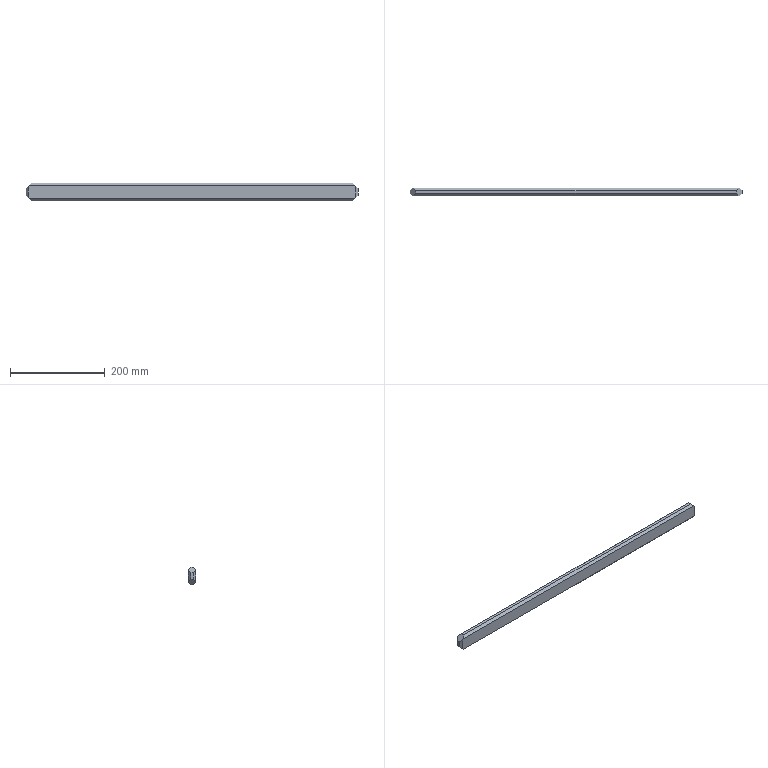Part | SolidWorks | features Chamfer 2, FlatPattern 1, SMBaseFlange 1, SheetMetal 1 | 1 solid | 18 faces | box 700 x 16 x 37 mm | volume 375009 mm3 | plane 18
STEP:
#1=CARTESIAN_POINT('',(0.,-11.,-25.));
#2=VERTEX_POINT('',#1);
#3=CARTESIAN_POINT('',(0.,-11.,-12.));
#4=VERTEX_POINT('',#3);
#5=CARTESIAN_POINT('',(0.,-11.,0.));
#6=DIRECTION('',(0.,0.,1.));
#7=VECTOR('',#6,1000.);
#8=LINE('',#5,#7);
#9=EDGE_CURVE('',#2,#4,#8,.T.);
#10=ORIENTED_EDGE('',*,*,#9,.T.);
#11=CARTESIAN_POINT('',(0.,-5.,-12.));
#12=VERTEX_POINT('',#11);
#13=CARTESIAN_POINT('',(0.,-16.,-12.));
#14=DIRECTION('',(0.,1.,0.));
#15=VECTOR('',#14,1000.);
#16=LINE('',#13,#15);
#17=EDGE_CURVE('',#4,#12,#16,.T.);
#18=ORIENTED_EDGE('',*,*,#17,.T.);
#19=CARTESIAN_POINT('',(0.,-5.,-25.));
#20=VERTEX_POINT('',#19);
#21=CARTESIAN_POINT('',(0.,-5.,-37.));
#22=DIRECTION('',(0.,0.,-1.));
#23=VECTOR('',#22,1000.);
#24=LINE('',#21,#23);
#25=EDGE_CURVE('',#12,#20,#24,.T.);
#26=ORIENTED_EDGE('',*,*,#25,.T.);
#27=CARTESIAN_POINT('',(0.,-16.,-25.));
#28=DIRECTION('',(0.,-1.,0.));
#29=VECTOR('',#28,1000.);
#30=LINE('',#27,#29);
#31=EDGE_CURVE('',#20,#2,#30,.T.);
#32=ORIENTED_EDGE('',*,*,#31,.T.);
#33=EDGE_LOOP('',(#10,#18,#26,#32));
#34=FACE_OUTER_BOUND('',#33,.T.);
#35=CARTESIAN_POINT('',(0.,-16.,0.));
#36=DIRECTION('',(-1.,0.,0.));
#37=DIRECTION('',(0.,0.,1.));
#38=AXIS2_PLACEMENT_3D('',#35,#36,#37);
#39=PLANE('',#38);
#40=ADVANCED_FACE('',(#34),#39,.T.);
#41=CARTESIAN_POINT('',(12.,-5.,-37.));
#42=VERTEX_POINT('',#41);
#43=CARTESIAN_POINT('',(688.,-5.,-37.));
#44=VERTEX_POINT('',#43);
#45=CARTESIAN_POINT('',(700.,-5.,-37.));
#46=DIRECTION('',(1.,0.,0.));
#47=VECTOR('',#46,1000.);
#48=LINE('',#45,#47);
#49=EDGE_CURVE('',#42,#44,#48,.T.);
#50=ORIENTED_EDGE('',*,*,#49,.T.);
#51=CARTESIAN_POINT('',(688.,-11.,-37.));
#52=VERTEX_POINT('',#51);
#53=CARTESIAN_POINT('',(688.,-16.,-37.));
#54=DIRECTION('',(0.,-1.,0.));
#55=VECTOR('',#54,1000.);
#56=LINE('',#53,#55);
#57=EDGE_CURVE('',#44,#52,#56,.T.);
#58=ORIENTED_EDGE('',*,*,#57,.T.);
#59=CARTESIAN_POINT('',(12.,-11.,-37.));
#60=VERTEX_POINT('',#59);
#61=CARTESIAN_POINT('',(0.,-11.,-37.));
#62=DIRECTION('',(-1.,0.,0.));
#63=VECTOR('',#62,1000.);
#64=LINE('',#61,#63);
#65=EDGE_CURVE('',#52,#60,#64,.T.);
#66=ORIENTED_EDGE('',*,*,#65,.T.);
#67=CARTESIAN_POINT('',(12.,-16.,-37.));
#68=DIRECTION('',(0.,1.,0.));
#69=VECTOR('',#68,1000.);
#70=LINE('',#67,#69);
#71=EDGE_CURVE('',#60,#42,#70,.T.);
#72=ORIENTED_EDGE('',*,*,#71,.T.);
#73=EDGE_LOOP('',(#50,#58,#66,#72));
#74=FACE_OUTER_BOUND('',#73,.T.);
#75=CARTESIAN_POINT('',(0.,-16.,-37.));
#76=DIRECTION('',(0.,0.,-1.));
#77=DIRECTION('',(-1.,0.,0.));
#78=AXIS2_PLACEMENT_3D('',#75,#76,#77);
#79=PLANE('',#78);
#80=ADVANCED_FACE('',(#74),#79,.T.);
#81=CARTESIAN_POINT('',(700.,-5.,-25.));
#82=VERTEX_POINT('',#81);
#83=CARTESIAN_POINT('',(700.,-5.,-12.));
#84=VERTEX_POINT('',#83);
#85=CARTESIAN_POINT('',(700.,-5.,0.));
#86=DIRECTION('',(0.,0.,1.));
#87=VECTOR('',#86,1000.);
#88=LINE('',#85,#87);
#89=EDGE_CURVE('',#82,#84,#88,.T.);
#90=ORIENTED_EDGE('',*,*,#89,.T.);
#91=CARTESIAN_POINT('',(700.,-11.,-12.));
#92=VERTEX_POINT('',#91);
#93=CARTESIAN_POINT('',(700.,-16.,-12.));
#94=DIRECTION('',(0.,-1.,0.));
#95=VECTOR('',#94,1000.);
#96=LINE('',#93,#95);
#97=EDGE_CURVE('',#84,#92,#96,.T.);
#98=ORIENTED_EDGE('',*,*,#97,.T.);
#99=CARTESIAN_POINT('',(700.,-11.,-25.));
#100=VERTEX_POINT('',#99);
#101=CARTESIAN_POINT('',(700.,-11.,0.));
#102=DIRECTION('',(0.,0.,-1.));
#103=VECTOR('',#102,1000.);
#104=LINE('',#101,#103);
#105=EDGE_CURVE('',#92,#100,#104,.T.);
#106=ORIENTED_EDGE('',*,*,#105,.T.);
#107=CARTESIAN_POINT('',(700.,-16.,-25.));
#108=DIRECTION('',(0.,1.,0.));
#109=VECTOR('',#108,1000.);
#110=LINE('',#107,#109);
#111=EDGE_CURVE('',#100,#82,#110,.T.);
#112=ORIENTED_EDGE('',*,*,#111,.T.);
#113=EDGE_LOOP('',(#90,#98,#106,#112));
#114=FACE_OUTER_BOUND('',#113,.T.);
#115=CARTESIAN_POINT('',(700.,-16.,0.));
#116=DIRECTION('',(1.,0.,0.));
#117=DIRECTION('',(0.,0.,-1.));
#118=AXIS2_PLACEMENT_3D('',#115,#116,#117);
#119=PLANE('',#118);
#120=ADVANCED_FACE('',(#114),#119,.T.);
#121=CARTESIAN_POINT('',(12.,-11.,0.));
#122=VERTEX_POINT('',#121);
#123=CARTESIAN_POINT('',(688.,-11.,0.));
#124=VERTEX_POINT('',#123);
#125=CARTESIAN_POINT('',(0.,-11.,0.));
#126=DIRECTION('',(1.,0.,0.));
#127=VECTOR('',#126,1000.);
#128=LINE('',#125,#127);
#129=EDGE_CURVE('',#122,#124,#128,.T.);
#130=ORIENTED_EDGE('',*,*,#129,.T.);
#131=CARTESIAN_POINT('',(688.,-5.,0.));
#132=VERTEX_POINT('',#131);
#133=CARTESIAN_POINT('',(688.,-16.,0.));
#134=DIRECTION('',(0.,1.,0.));
#135=VECTOR('',#134,1000.);
#136=LINE('',#133,#135);
#137=EDGE_CURVE('',#124,#132,#136,.T.);
#138=ORIENTED_EDGE('',*,*,#137,.T.);
#139=CARTESIAN_POINT('',(12.,-5.,0.));
#140=VERTEX_POINT('',#139);
#141=CARTESIAN_POINT('',(0.,-5.,0.));
#142=DIRECTION('',(-1.,0.,0.));
#143=VECTOR('',#142,1000.);
#144=LINE('',#141,#143);
#145=EDGE_CURVE('',#132,#140,#144,.T.);
#146=ORIENTED_EDGE('',*,*,#145,.T.);
#147=CARTESIAN_POINT('',(12.,-16.,0.));
#148=DIRECTION('',(0.,-1.,0.));
#149=VECTOR('',#148,1000.);
#150=LINE('',#147,#149);
#151=EDGE_CURVE('',#140,#122,#150,.T.);
#152=ORIENTED_EDGE('',*,*,#151,.T.);
#153=EDGE_LOOP('',(#130,#138,#146,#152));
#154=FACE_OUTER_BOUND('',#153,.T.);
#155=CARTESIAN_POINT('',(0.,-16.,0.));
#156=DIRECTION('',(0.,0.,1.));
#157=DIRECTION('',(1.,0.,0.));
#158=AXIS2_PLACEMENT_3D('',#155,#156,#157);
#159=PLANE('',#158);
#160=ADVANCED_FACE('',(#154),#159,.T.);
#161=CARTESIAN_POINT('',(695.,-16.,-30.));
#162=VERTEX_POINT('',#161);
#163=CARTESIAN_POINT('',(695.,-16.,-7.));
#164=VERTEX_POINT('',#163);
#165=CARTESIAN_POINT('',(695.,-16.,-37.));
#166=DIRECTION('',(0.,0.,1.));
#167=VECTOR('',#166,1000.);
#168=LINE('',#165,#167);
#169=EDGE_CURVE('',#162,#164,#168,.T.);
#170=ORIENTED_EDGE('',*,*,#169,.T.);
#171=CARTESIAN_POINT('',(693.,-16.,-5.));
#172=VERTEX_POINT('',#171);
#173=CARTESIAN_POINT('',(362.5,-16.,325.5));
#174=DIRECTION('',(-0.7071,0.,0.7071));
#175=VECTOR('',#174,1000.);
#176=LINE('',#173,#175);
#177=EDGE_CURVE('',#164,#172,#176,.T.);
#178=ORIENTED_EDGE('',*,*,#177,.T.);
#179=CARTESIAN_POINT('',(7.,-16.,-5.));
#180=VERTEX_POINT('',#179);
#181=CARTESIAN_POINT('',(0.,-16.,-5.));
#182=DIRECTION('',(-1.,0.,0.));
#183=VECTOR('',#182,1000.);
#184=LINE('',#181,#183);
#185=EDGE_CURVE('',#172,#180,#184,.T.);
#186=ORIENTED_EDGE('',*,*,#185,.T.);
#187=CARTESIAN_POINT('',(5.,-16.,-7.));
#188=VERTEX_POINT('',#187);
#189=CARTESIAN_POINT('',(-12.5,-16.,-24.5));
#190=DIRECTION('',(-0.7071,0.,-0.7071));
#191=VECTOR('',#190,1000.);
#192=LINE('',#189,#191);
#193=EDGE_CURVE('',#180,#188,#192,.T.);
#194=ORIENTED_EDGE('',*,*,#193,.T.);
#195=CARTESIAN_POINT('',(5.,-16.,-30.));
#196=VERTEX_POINT('',#195);
#197=CARTESIAN_POINT('',(5.,-16.,-37.));
#198=DIRECTION('',(0.,0.,-1.));
#199=VECTOR('',#198,1000.);
#200=LINE('',#197,#199);
#201=EDGE_CURVE('',#188,#196,#200,.T.);
#202=ORIENTED_EDGE('',*,*,#201,.T.);
#203=CARTESIAN_POINT('',(7.,-16.,-32.));
#204=VERTEX_POINT('',#203);
#205=CARTESIAN_POINT('',(6.,-16.,-31.));
#206=DIRECTION('',(0.7071,0.,-0.7071));
#207=VECTOR('',#206,1000.);
#208=LINE('',#205,#207);
#209=EDGE_CURVE('',#196,#204,#208,.T.);
#210=ORIENTED_EDGE('',*,*,#209,.T.);
#211=CARTESIAN_POINT('',(693.,-16.,-32.));
#212=VERTEX_POINT('',#211);
#213=CARTESIAN_POINT('',(0.,-16.,-32.));
#214=DIRECTION('',(1.,0.,0.));
#215=VECTOR('',#214,1000.);
#216=LINE('',#213,#215);
#217=EDGE_CURVE('',#204,#212,#216,.T.);
#218=ORIENTED_EDGE('',*,*,#217,.T.);
#219=CARTESIAN_POINT('',(344.,-16.,-381.));
#220=DIRECTION('',(0.7071,0.,0.7071));
#221=VECTOR('',#220,1000.);
#222=LINE('',#219,#221);
#223=EDGE_CURVE('',#212,#162,#222,.T.);
#224=ORIENTED_EDGE('',*,*,#223,.T.);
#225=EDGE_LOOP('',(#170,#178,#186,#194,#202,#210,#218,#224));
#226=FACE_OUTER_BOUND('',#225,.T.);
#227=CARTESIAN_POINT('',(0.,-16.,-37.));
#228=DIRECTION('',(0.,-1.,0.));
#229=DIRECTION('',(0.,0.,-1.));
#230=AXIS2_PLACEMENT_3D('',#227,#228,#229);
#231=PLANE('',#230);
#232=ADVANCED_FACE('',(#226),#231,.T.);
#233=CARTESIAN_POINT('',(7.,0.,-5.));
#234=VERTEX_POINT('',#233);
#235=CARTESIAN_POINT('',(693.,0.,-5.));
#236=VERTEX_POINT('',#235);
#237=CARTESIAN_POINT('',(700.,0.,-5.));
#238=DIRECTION('',(1.,0.,0.));
#239=VECTOR('',#238,1000.);
#240=LINE('',#237,#239);
#241=EDGE_CURVE('',#234,#236,#240,.T.);
#242=ORIENTED_EDGE('',*,*,#241,.T.);
#243=CARTESIAN_POINT('',(695.,0.,-7.));
#244=VERTEX_POINT('',#243);
#245=CARTESIAN_POINT('',(688.,0.,0.));
#246=DIRECTION('',(0.7071,0.,-0.7071));
#247=VECTOR('',#246,1000.);
#248=LINE('',#245,#247);
#249=EDGE_CURVE('',#236,#244,#248,.T.);
#250=ORIENTED_EDGE('',*,*,#249,.T.);
#251=CARTESIAN_POINT('',(695.,0.,-30.));
#252=VERTEX_POINT('',#251);
#253=CARTESIAN_POINT('',(695.,0.,-37.));
#254=DIRECTION('',(0.,0.,-1.));
#255=VECTOR('',#254,1000.);
#256=LINE('',#253,#255);
#257=EDGE_CURVE('',#244,#252,#256,.T.);
#258=ORIENTED_EDGE('',*,*,#257,.T.);
#259=CARTESIAN_POINT('',(693.,0.,-32.));
#260=VERTEX_POINT('',#259);
#261=CARTESIAN_POINT('',(700.,0.,-25.));
#262=DIRECTION('',(-0.7071,0.,-0.7071));
#263=VECTOR('',#262,1000.);
#264=LINE('',#261,#263);
#265=EDGE_CURVE('',#252,#260,#264,.T.);
#266=ORIENTED_EDGE('',*,*,#265,.T.);
#267=CARTESIAN_POINT('',(7.,0.,-32.));
#268=VERTEX_POINT('',#267);
#269=CARTESIAN_POINT('',(0.,0.,-32.));
#270=DIRECTION('',(-1.,0.,0.));
#271=VECTOR('',#270,1000.);
#272=LINE('',#269,#271);
#273=EDGE_CURVE('',#260,#268,#272,.T.);
#274=ORIENTED_EDGE('',*,*,#273,.T.);
#275=CARTESIAN_POINT('',(5.,0.,-30.));
#276=VERTEX_POINT('',#275);
#277=CARTESIAN_POINT('',(12.,0.,-37.));
#278=DIRECTION('',(-0.7071,0.,0.7071));
#279=VECTOR('',#278,1000.);
#280=LINE('',#277,#279);
#281=EDGE_CURVE('',#268,#276,#280,.T.);
#282=ORIENTED_EDGE('',*,*,#281,.T.);
#283=CARTESIAN_POINT('',(5.,0.,-7.));
#284=VERTEX_POINT('',#283);
#285=CARTESIAN_POINT('',(5.,0.,0.));
#286=DIRECTION('',(0.,0.,1.));
#287=VECTOR('',#286,1000.);
#288=LINE('',#285,#287);
#289=EDGE_CURVE('',#276,#284,#288,.T.);
#290=ORIENTED_EDGE('',*,*,#289,.T.);
#291=CARTESIAN_POINT('',(0.,0.,-12.));
#292=DIRECTION('',(0.7071,0.,0.7071));
#293=VECTOR('',#292,1000.);
#294=LINE('',#291,#293);
#295=EDGE_CURVE('',#284,#234,#294,.T.);
#296=ORIENTED_EDGE('',*,*,#295,.T.);
#297=EDGE_LOOP('',(#242,#250,#258,#266,#274,#282,#290,#296));
#298=FACE_OUTER_BOUND('',#297,.T.);
#299=CARTESIAN_POINT('',(0.,0.,-37.));
#300=DIRECTION('',(0.,-1.,0.));
#301=DIRECTION('',(0.,0.,-1.));
#302=AXIS2_PLACEMENT_3D('',#299,#300,#301);
#303=PLANE('',#302);
#304=ADVANCED_FACE('',(#298),#303,.F.);
#305=ORIENTED_EDGE('',*,*,#201,.F.);
#306=CARTESIAN_POINT('',(4.,-15.,-8.));
#307=DIRECTION('',(-0.5774,0.5774,-0.5774));
#308=VECTOR('',#307,1000.);
#309=LINE('',#306,#308);
#310=EDGE_CURVE('',#188,#4,#309,.T.);
#311=ORIENTED_EDGE('',*,*,#310,.T.);
#312=ORIENTED_EDGE('',*,*,#9,.F.);
#313=CARTESIAN_POINT('',(-8.333,-2.667,-16.667));
#314=DIRECTION('',(0.5774,-0.5774,-0.5774));
#315=VECTOR('',#314,1000.);
#316=LINE('',#313,#315);
#317=EDGE_CURVE('',#2,#196,#316,.T.);
#318=ORIENTED_EDGE('',*,*,#317,.T.);
#319=EDGE_LOOP('',(#305,#311,#312,#318));
#320=FACE_OUTER_BOUND('',#319,.T.);
#321=CARTESIAN_POINT('',(0.,-11.,0.));
#322=DIRECTION('',(0.7071,0.7071,0.));
#323=DIRECTION('',(-0.7071,0.7071,0.));
#324=AXIS2_PLACEMENT_3D('',#321,#322,#323);
#325=PLANE('',#324);
#326=ADVANCED_FACE('',(#320),#325,.F.);
#327=ORIENTED_EDGE('',*,*,#185,.F.);
#328=CARTESIAN_POINT('',(458.667,218.333,229.333));
#329=DIRECTION('',(-0.5774,0.5774,0.5774));
#330=VECTOR('',#329,1000.);
#331=LINE('',#328,#330);
#332=EDGE_CURVE('',#172,#124,#331,.T.);
#333=ORIENTED_EDGE('',*,*,#332,.T.);
#334=ORIENTED_EDGE('',*,*,#129,.F.);
#335=CARTESIAN_POINT('',(8.,-15.,-4.));
#336=DIRECTION('',(-0.5774,-0.5774,-0.5774));
#337=VECTOR('',#336,1000.);
#338=LINE('',#335,#337);
#339=EDGE_CURVE('',#122,#180,#338,.T.);
#340=ORIENTED_EDGE('',*,*,#339,.T.);
#341=EDGE_LOOP('',(#327,#333,#334,#340));
#342=FACE_OUTER_BOUND('',#341,.T.);
#343=CARTESIAN_POINT('',(0.,-11.,0.));
#344=DIRECTION('',(0.,0.7071,-0.7071));
#345=DIRECTION('',(0.,0.7071,0.7071));
#346=AXIS2_PLACEMENT_3D('',#343,#344,#345);
#347=PLANE('',#346);
#348=ADVANCED_FACE('',(#342),#347,.F.);
#349=ORIENTED_EDGE('',*,*,#65,.F.);
#350=CARTESIAN_POINT('',(458.667,218.333,-266.333));
#351=DIRECTION('',(0.5774,-0.5774,0.5774));
#352=VECTOR('',#351,1000.);
#353=LINE('',#350,#352);
#354=EDGE_CURVE('',#52,#212,#353,.T.);
#355=ORIENTED_EDGE('',*,*,#354,.T.);
#356=ORIENTED_EDGE('',*,*,#217,.F.);
#357=CARTESIAN_POINT('',(8.,-15.,-33.));
#358=DIRECTION('',(0.5774,0.5774,-0.5774));
#359=VECTOR('',#358,1000.);
#360=LINE('',#357,#359);
#361=EDGE_CURVE('',#204,#60,#360,.T.);
#362=ORIENTED_EDGE('',*,*,#361,.T.);
#363=EDGE_LOOP('',(#349,#355,#356,#362));
#364=FACE_OUTER_BOUND('',#363,.T.);
#365=CARTESIAN_POINT('',(0.,-11.,-37.));
#366=DIRECTION('',(0.,0.7071,0.7071));
#367=DIRECTION('',(0.,-0.7071,0.7071));
#368=AXIS2_PLACEMENT_3D('',#365,#366,#367);
#369=PLANE('',#368);
#370=ADVANCED_FACE('',(#364),#369,.F.);
#371=ORIENTED_EDGE('',*,*,#105,.F.);
#372=CARTESIAN_POINT('',(696.,-15.,-8.));
#373=DIRECTION('',(-0.5774,-0.5774,0.5774));
#374=VECTOR('',#373,1000.);
#375=LINE('',#372,#374);
#376=EDGE_CURVE('',#92,#164,#375,.T.);
#377=ORIENTED_EDGE('',*,*,#376,.T.);
#378=ORIENTED_EDGE('',*,*,#169,.F.);
#379=CARTESIAN_POINT('',(708.333,-2.667,-16.667));
#380=DIRECTION('',(0.5774,0.5774,0.5774));
#381=VECTOR('',#380,1000.);
#382=LINE('',#379,#381);
#383=EDGE_CURVE('',#162,#100,#382,.T.);
#384=ORIENTED_EDGE('',*,*,#383,.T.);
#385=EDGE_LOOP('',(#371,#377,#378,#384));
#386=FACE_OUTER_BOUND('',#385,.T.);
#387=CARTESIAN_POINT('',(700.,-11.,0.));
#388=DIRECTION('',(-0.7071,0.7071,0.));
#389=DIRECTION('',(-0.7071,-0.7071,0.));
#390=AXIS2_PLACEMENT_3D('',#387,#388,#389);
#391=PLANE('',#390);
#392=ADVANCED_FACE('',(#386),#391,.F.);
#393=ORIENTED_EDGE('',*,*,#25,.F.);
#394=CARTESIAN_POINT('',(-5.,-10.,-17.));
#395=DIRECTION('',(0.5774,0.5774,0.5774));
#396=VECTOR('',#395,1000.);
#397=LINE('',#394,#396);
#398=EDGE_CURVE('',#12,#284,#397,.T.);
#399=ORIENTED_EDGE('',*,*,#398,.T.);
#400=ORIENTED_EDGE('',*,*,#289,.F.);
#401=CARTESIAN_POINT('',(7.333,2.333,-32.333));
#402=DIRECTION('',(-0.5774,-0.5774,0.5774));
#403=VECTOR('',#402,1000.);
#404=LINE('',#401,#403);
#405=EDGE_CURVE('',#276,#20,#404,.T.);
#406=ORIENTED_EDGE('',*,*,#405,.T.);
#407=EDGE_LOOP('',(#393,#399,#400,#406));
#408=FACE_OUTER_BOUND('',#407,.T.);
#409=CARTESIAN_POINT('',(5.,0.,-37.));
#410=DIRECTION('',(-0.7071,0.7071,0.));
#411=DIRECTION('',(-0.7071,-0.7071,0.));
#412=AXIS2_PLACEMENT_3D('',#409,#410,#411);
#413=PLANE('',#412);
#414=ADVANCED_FACE('',(#408),#413,.T.);
#415=ORIENTED_EDGE('',*,*,#145,.F.);
#416=CARTESIAN_POINT('',(462.,-231.,226.));
#417=DIRECTION('',(0.5774,0.5774,-0.5774));
#418=VECTOR('',#417,1000.);
#419=LINE('',#416,#418);
#420=EDGE_CURVE('',#132,#236,#419,.T.);
#421=ORIENTED_EDGE('',*,*,#420,.T.);
#422=ORIENTED_EDGE('',*,*,#241,.F.);
#423=CARTESIAN_POINT('',(4.667,2.333,-7.333));
#424=DIRECTION('',(0.5774,-0.5774,0.5774));
#425=VECTOR('',#424,1000.);
#426=LINE('',#423,#425);
#427=EDGE_CURVE('',#234,#140,#426,.T.);
#428=ORIENTED_EDGE('',*,*,#427,.T.);
#429=EDGE_LOOP('',(#415,#421,#422,#428));
#430=FACE_OUTER_BOUND('',#429,.T.);
#431=CARTESIAN_POINT('',(0.,0.,-5.));
#432=DIRECTION('',(0.,0.7071,0.7071));
#433=DIRECTION('',(0.,-0.7071,0.7071));
#434=AXIS2_PLACEMENT_3D('',#431,#432,#433);
#435=PLANE('',#434);
#436=ADVANCED_FACE('',(#430),#435,.T.);
#437=ORIENTED_EDGE('',*,*,#273,.F.);
#438=CARTESIAN_POINT('',(462.,-231.,-263.));
#439=DIRECTION('',(-0.5774,-0.5774,-0.5774));
#440=VECTOR('',#439,1000.);
#441=LINE('',#438,#440);
#442=EDGE_CURVE('',#260,#44,#441,.T.);
#443=ORIENTED_EDGE('',*,*,#442,.T.);
#444=ORIENTED_EDGE('',*,*,#49,.F.);
#445=CARTESIAN_POINT('',(4.667,2.333,-29.667));
#446=DIRECTION('',(-0.5774,0.5774,0.5774));
#447=VECTOR('',#446,1000.);
#448=LINE('',#445,#447);
#449=EDGE_CURVE('',#42,#268,#448,.T.);
#450=ORIENTED_EDGE('',*,*,#449,.T.);
#451=EDGE_LOOP('',(#437,#443,#444,#450));
#452=FACE_OUTER_BOUND('',#451,.T.);
#453=CARTESIAN_POINT('',(0.,0.,-32.));
#454=DIRECTION('',(0.,0.7071,-0.7071));
#455=DIRECTION('',(0.,0.7071,0.7071));
#456=AXIS2_PLACEMENT_3D('',#453,#454,#455);
#457=PLANE('',#456);
#458=ADVANCED_FACE('',(#452),#457,.T.);
#459=ORIENTED_EDGE('',*,*,#257,.F.);
#460=CARTESIAN_POINT('',(705.,-10.,-17.));
#461=DIRECTION('',(0.5774,-0.5774,-0.5774));
#462=VECTOR('',#461,1000.);
#463=LINE('',#460,#462);
#464=EDGE_CURVE('',#244,#84,#463,.T.);
#465=ORIENTED_EDGE('',*,*,#464,.T.);
#466=ORIENTED_EDGE('',*,*,#89,.F.);
#467=CARTESIAN_POINT('',(692.667,2.333,-32.333));
#468=DIRECTION('',(-0.5774,0.5774,-0.5774));
#469=VECTOR('',#468,1000.);
#470=LINE('',#467,#469);
#471=EDGE_CURVE('',#82,#252,#470,.T.);
#472=ORIENTED_EDGE('',*,*,#471,.T.);
#473=EDGE_LOOP('',(#459,#465,#466,#472));
#474=FACE_OUTER_BOUND('',#473,.T.);
#475=CARTESIAN_POINT('',(695.,0.,-37.));
#476=DIRECTION('',(0.7071,0.7071,0.));
#477=DIRECTION('',(-0.7071,0.7071,0.));
#478=AXIS2_PLACEMENT_3D('',#475,#476,#477);
#479=PLANE('',#478);
#480=ADVANCED_FACE('',(#474),#479,.T.);
#481=ORIENTED_EDGE('',*,*,#376,.F.);
#482=ORIENTED_EDGE('',*,*,#97,.F.);
#483=ORIENTED_EDGE('',*,*,#464,.F.);
#484=ORIENTED_EDGE('',*,*,#249,.F.);
#485=ORIENTED_EDGE('',*,*,#420,.F.);
#486=ORIENTED_EDGE('',*,*,#137,.F.);
#487=ORIENTED_EDGE('',*,*,#332,.F.);
#488=ORIENTED_EDGE('',*,*,#177,.F.);
#489=EDGE_LOOP('',(#481,#482,#483,#484,#485,#486,#487,#488));
#490=FACE_OUTER_BOUND('',#489,.T.);
#491=CARTESIAN_POINT('',(688.,-16.,0.));
#492=DIRECTION('',(-0.7071,0.,-0.7071));
#493=DIRECTION('',(-0.7071,0.,0.7071));
#494=AXIS2_PLACEMENT_3D('',#491,#492,#493);
#495=PLANE('',#494);
#496=ADVANCED_FACE('',(#490),#495,.F.);
#497=ORIENTED_EDGE('',*,*,#354,.F.);
#498=ORIENTED_EDGE('',*,*,#57,.F.);
#499=ORIENTED_EDGE('',*,*,#442,.F.);
#500=ORIENTED_EDGE('',*,*,#265,.F.);
#501=ORIENTED_EDGE('',*,*,#471,.F.);
#502=ORIENTED_EDGE('',*,*,#111,.F.);
#503=ORIENTED_EDGE('',*,*,#383,.F.);
#504=ORIENTED_EDGE('',*,*,#223,.F.);
#505=EDGE_LOOP('',(#497,#498,#499,#500,#501,#502,#503,#504));
#506=FACE_OUTER_BOUND('',#505,.T.);
#507=CARTESIAN_POINT('',(700.,-16.,-25.));
#508=DIRECTION('',(-0.7071,0.,0.7071));
#509=DIRECTION('',(0.7071,0.,0.7071));
#510=AXIS2_PLACEMENT_3D('',#507,#508,#509);
#511=PLANE('',#510);
#512=ADVANCED_FACE('',(#506),#511,.F.);
#513=ORIENTED_EDGE('',*,*,#339,.F.);
#514=ORIENTED_EDGE('',*,*,#151,.F.);
#515=ORIENTED_EDGE('',*,*,#427,.F.);
#516=ORIENTED_EDGE('',*,*,#295,.F.);
#517=ORIENTED_EDGE('',*,*,#398,.F.);
#518=ORIENTED_EDGE('',*,*,#17,.F.);
#519=ORIENTED_EDGE('',*,*,#310,.F.);
#520=ORIENTED_EDGE('',*,*,#193,.F.);
#521=EDGE_LOOP('',(#513,#514,#515,#516,#517,#518,#519,#520));
#522=FACE_OUTER_BOUND('',#521,.T.);
#523=CARTESIAN_POINT('',(0.,-16.,-12.));
#524=DIRECTION('',(0.7071,0.,-0.7071));
#525=DIRECTION('',(-0.7071,0.,-0.7071));
#526=AXIS2_PLACEMENT_3D('',#523,#524,#525);
#527=PLANE('',#526);
#528=ADVANCED_FACE('',(#522),#527,.F.);
#529=ORIENTED_EDGE('',*,*,#317,.F.);
#530=ORIENTED_EDGE('',*,*,#31,.F.);
#531=ORIENTED_EDGE('',*,*,#405,.F.);
#532=ORIENTED_EDGE('',*,*,#281,.F.);
#533=ORIENTED_EDGE('',*,*,#449,.F.);
#534=ORIENTED_EDGE('',*,*,#71,.F.);
#535=ORIENTED_EDGE('',*,*,#361,.F.);
#536=ORIENTED_EDGE('',*,*,#209,.F.);
#537=EDGE_LOOP('',(#529,#530,#531,#532,#533,#534,#535,#536));
#538=FACE_OUTER_BOUND('',#537,.T.);
#539=CARTESIAN_POINT('',(12.,-16.,-37.));
#540=DIRECTION('',(0.7071,0.,0.7071));
#541=DIRECTION('',(0.7071,0.,-0.7071));
#542=AXIS2_PLACEMENT_3D('',#539,#540,#541);
#543=PLANE('',#542);
#544=ADVANCED_FACE('',(#538),#543,.F.);
#545=CLOSED_SHELL('',(#40,#80,#120,#160,#232,#304,#326,#348,#370,#392,#414,#436,#458,#480,#496,#512,#528,#544));
#546=MANIFOLD_SOLID_BREP('',#545);
#547=CARTESIAN_POINT('',(0.,0.,0.));
#548=DIRECTION('',(0.,0.,1.));
#549=DIRECTION('',(1.,0.,0.));
#550=AXIS2_PLACEMENT_3D('',#547,#548,#549);
#551=(LENGTH_UNIT()NAMED_UNIT(*)SI_UNIT(.MILLI.,.METRE.));
#552=UNCERTAINTY_MEASURE_WITH_UNIT(LENGTH_MEASURE(0.00001),#551,'','');
#553=(NAMED_UNIT(*)PLANE_ANGLE_UNIT()SI_UNIT($,.RADIAN.));
#554=(NAMED_UNIT(*)SI_UNIT($,.STERADIAN.)SOLID_ANGLE_UNIT());
#555=(GEOMETRIC_REPRESENTATION_CONTEXT(3)GLOBAL_UNCERTAINTY_ASSIGNED_CONTEXT((#552))GLOBAL_UNIT_ASSIGNED_CONTEXT((#551,#553,#554))REPRESENTATION_CONTEXT('',''));
#556=ADVANCED_BREP_SHAPE_REPRESENTATION('',(#546,#550),#555);